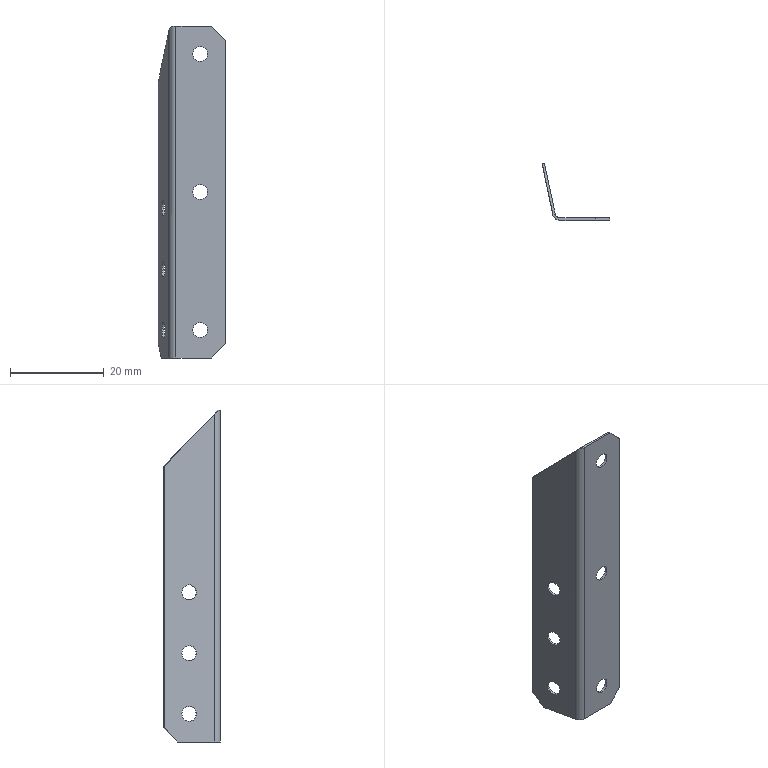Part | SolidWorks | features BaseBody 1 | 1 solid | 27 faces | box 14.467 x 12.157 x 71 mm | volume 767.375 mm3 | cylinder 14 | plane 12 | spline 1 | commonest cylinder face diameters 3.2 x12 2 x1 3 x1
STEP:
#1=CARTESIAN_POINT('',(6.25,-0.5,-27.9));
#2=VERTEX_POINT('',#1);
#3=CARTESIAN_POINT('',(6.25,-0.5,-31.1));
#4=VERTEX_POINT('',#3);
#5=CARTESIAN_POINT('',(6.25,-0.5,-29.5));
#6=DIRECTION('',(0.,-1.,0.));
#7=DIRECTION('',(0.,0.,1.));
#8=AXIS2_PLACEMENT_3D('',#5,#6,#7);
#9=CIRCLE('',#8,1.6);
#10=EDGE_CURVE('',#2,#4,#9,.T.);
#11=ORIENTED_EDGE('',*,*,#10,.T.);
#12=CARTESIAN_POINT('',(6.25,0.,-31.1));
#13=VERTEX_POINT('',#12);
#14=CARTESIAN_POINT('',(6.25,-0.5,-31.1));
#15=DIRECTION('',(0.,1.,0.));
#16=VECTOR('',#15,1000.);
#17=LINE('',#14,#16);
#18=EDGE_CURVE('',#4,#13,#17,.T.);
#19=ORIENTED_EDGE('',*,*,#18,.T.);
#20=CARTESIAN_POINT('',(6.25,0.,-27.9));
#21=VERTEX_POINT('',#20);
#22=CARTESIAN_POINT('',(6.25,0.,-29.5));
#23=DIRECTION('',(0.,1.,0.));
#24=DIRECTION('',(0.,0.,1.));
#25=AXIS2_PLACEMENT_3D('',#22,#23,#24);
#26=CIRCLE('',#25,1.6);
#27=EDGE_CURVE('',#13,#21,#26,.T.);
#28=ORIENTED_EDGE('',*,*,#27,.T.);
#29=CARTESIAN_POINT('',(6.25,-0.5,-27.9));
#30=DIRECTION('',(0.,1.,0.));
#31=VECTOR('',#30,1000.);
#32=LINE('',#29,#31);
#33=EDGE_CURVE('',#2,#21,#32,.T.);
#34=ORIENTED_EDGE('',*,*,#33,.F.);
#35=EDGE_LOOP('',(#11,#19,#28,#34));
#36=FACE_OUTER_BOUND('',#35,.T.);
#37=CARTESIAN_POINT('',(6.25,-0.5,-29.5));
#38=DIRECTION('',(0.,1.,0.));
#39=DIRECTION('',(0.,0.,1.));
#40=AXIS2_PLACEMENT_3D('',#37,#38,#39);
#41=CYLINDRICAL_SURFACE('',#40,1.6);
#42=ADVANCED_FACE('',(#36),#41,.F.);
#43=CARTESIAN_POINT('',(6.25,-0.5,1.6));
#44=VERTEX_POINT('',#43);
#45=CARTESIAN_POINT('',(6.25,-0.5,-1.6));
#46=VERTEX_POINT('',#45);
#47=CARTESIAN_POINT('',(6.25,-0.5,0.));
#48=DIRECTION('',(0.,-1.,0.));
#49=DIRECTION('',(0.,0.,1.));
#50=AXIS2_PLACEMENT_3D('',#47,#48,#49);
#51=CIRCLE('',#50,1.6);
#52=EDGE_CURVE('',#44,#46,#51,.T.);
#53=ORIENTED_EDGE('',*,*,#52,.T.);
#54=CARTESIAN_POINT('',(6.25,0.,-1.6));
#55=VERTEX_POINT('',#54);
#56=CARTESIAN_POINT('',(6.25,-0.5,-1.6));
#57=DIRECTION('',(0.,1.,0.));
#58=VECTOR('',#57,1000.);
#59=LINE('',#56,#58);
#60=EDGE_CURVE('',#46,#55,#59,.T.);
#61=ORIENTED_EDGE('',*,*,#60,.T.);
#62=CARTESIAN_POINT('',(6.25,0.,1.6));
#63=VERTEX_POINT('',#62);
#64=CARTESIAN_POINT('',(6.25,0.,0.));
#65=DIRECTION('',(0.,-1.,0.));
#66=DIRECTION('',(0.,0.,1.));
#67=AXIS2_PLACEMENT_3D('',#64,#65,#66);
#68=CIRCLE('',#67,1.6);
#69=EDGE_CURVE('',#63,#55,#68,.T.);
#70=ORIENTED_EDGE('',*,*,#69,.F.);
#71=CARTESIAN_POINT('',(6.25,-0.5,1.6));
#72=DIRECTION('',(0.,1.,0.));
#73=VECTOR('',#72,1000.);
#74=LINE('',#71,#73);
#75=EDGE_CURVE('',#44,#63,#74,.T.);
#76=ORIENTED_EDGE('',*,*,#75,.F.);
#77=EDGE_LOOP('',(#53,#61,#70,#76));
#78=FACE_OUTER_BOUND('',#77,.T.);
#79=CARTESIAN_POINT('',(6.25,-0.5,0.));
#80=DIRECTION('',(0.,1.,0.));
#81=DIRECTION('',(0.,0.,1.));
#82=AXIS2_PLACEMENT_3D('',#79,#80,#81);
#83=CYLINDRICAL_SURFACE('',#82,1.6);
#84=ADVANCED_FACE('',(#78),#83,.F.);
#85=CARTESIAN_POINT('',(6.25,-0.5,31.1));
#86=VERTEX_POINT('',#85);
#87=CARTESIAN_POINT('',(6.25,-0.5,27.9));
#88=VERTEX_POINT('',#87);
#89=CARTESIAN_POINT('',(6.25,-0.5,29.5));
#90=DIRECTION('',(0.,-1.,0.));
#91=DIRECTION('',(0.,0.,1.));
#92=AXIS2_PLACEMENT_3D('',#89,#90,#91);
#93=CIRCLE('',#92,1.6);
#94=EDGE_CURVE('',#86,#88,#93,.T.);
#95=ORIENTED_EDGE('',*,*,#94,.T.);
#96=CARTESIAN_POINT('',(6.25,0.,27.9));
#97=VERTEX_POINT('',#96);
#98=CARTESIAN_POINT('',(6.25,-0.5,27.9));
#99=DIRECTION('',(0.,1.,0.));
#100=VECTOR('',#99,1000.);
#101=LINE('',#98,#100);
#102=EDGE_CURVE('',#88,#97,#101,.T.);
#103=ORIENTED_EDGE('',*,*,#102,.T.);
#104=CARTESIAN_POINT('',(6.25,0.,31.1));
#105=VERTEX_POINT('',#104);
#106=CARTESIAN_POINT('',(6.25,0.,29.5));
#107=DIRECTION('',(0.,-1.,0.));
#108=DIRECTION('',(0.,0.,1.));
#109=AXIS2_PLACEMENT_3D('',#106,#107,#108);
#110=CIRCLE('',#109,1.6);
#111=EDGE_CURVE('',#105,#97,#110,.T.);
#112=ORIENTED_EDGE('',*,*,#111,.F.);
#113=CARTESIAN_POINT('',(6.25,-0.5,31.1));
#114=DIRECTION('',(0.,1.,0.));
#115=VECTOR('',#114,1000.);
#116=LINE('',#113,#115);
#117=EDGE_CURVE('',#86,#105,#116,.T.);
#118=ORIENTED_EDGE('',*,*,#117,.F.);
#119=EDGE_LOOP('',(#95,#103,#112,#118));
#120=FACE_OUTER_BOUND('',#119,.T.);
#121=CARTESIAN_POINT('',(6.25,-0.5,29.5));
#122=DIRECTION('',(0.,1.,0.));
#123=DIRECTION('',(0.,0.,1.));
#124=AXIS2_PLACEMENT_3D('',#121,#122,#123);
#125=CYLINDRICAL_SURFACE('',#124,1.6);
#126=ADVANCED_FACE('',(#120),#125,.F.);
#127=CARTESIAN_POINT('',(-1.906,7.739,-29.5));
#128=VERTEX_POINT('',#127);
#129=CARTESIAN_POINT('',(-1.241,4.609,-29.5));
#130=VERTEX_POINT('',#129);
#131=CARTESIAN_POINT('',(-1.573,6.174,-29.5));
#132=DIRECTION('',(-0.9781,-0.2079,0.));
#133=DIRECTION('',(-0.2079,0.9781,0.));
#134=AXIS2_PLACEMENT_3D('',#131,#132,#133);
#135=CIRCLE('',#134,1.6);
#136=EDGE_CURVE('',#128,#130,#135,.T.);
#137=ORIENTED_EDGE('',*,*,#136,.T.);
#138=CARTESIAN_POINT('',(-0.7517,4.713,-29.5));
#139=VERTEX_POINT('',#138);
#140=CARTESIAN_POINT('',(-1.241,4.609,-29.5));
#141=DIRECTION('',(0.9781,0.2079,0.));
#142=VECTOR('',#141,1000.);
#143=LINE('',#140,#142);
#144=EDGE_CURVE('',#130,#139,#143,.T.);
#145=ORIENTED_EDGE('',*,*,#144,.T.);
#146=CARTESIAN_POINT('',(-1.417,7.843,-29.5));
#147=VERTEX_POINT('',#146);
#148=CARTESIAN_POINT('',(-1.084,6.278,-29.5));
#149=DIRECTION('',(-0.9781,-0.2079,0.));
#150=DIRECTION('',(-0.2079,0.9781,0.));
#151=AXIS2_PLACEMENT_3D('',#148,#149,#150);
#152=CIRCLE('',#151,1.6);
#153=EDGE_CURVE('',#147,#139,#152,.T.);
#154=ORIENTED_EDGE('',*,*,#153,.F.);
#155=CARTESIAN_POINT('',(-1.906,7.739,-29.5));
#156=DIRECTION('',(0.9781,0.2079,0.));
#157=VECTOR('',#156,1000.);
#158=LINE('',#155,#157);
#159=EDGE_CURVE('',#128,#147,#158,.T.);
#160=ORIENTED_EDGE('',*,*,#159,.F.);
#161=EDGE_LOOP('',(#137,#145,#154,#160));
#162=FACE_OUTER_BOUND('',#161,.T.);
#163=CARTESIAN_POINT('',(-1.573,6.174,-29.5));
#164=DIRECTION('',(0.9781,0.2079,0.));
#165=DIRECTION('',(-0.2079,0.9781,0.));
#166=AXIS2_PLACEMENT_3D('',#163,#164,#165);
#167=CYLINDRICAL_SURFACE('',#166,1.6);
#168=ADVANCED_FACE('',(#162),#167,.F.);
#169=CARTESIAN_POINT('',(-1.906,7.739,-16.5));
#170=VERTEX_POINT('',#169);
#171=CARTESIAN_POINT('',(-1.241,4.609,-16.5));
#172=VERTEX_POINT('',#171);
#173=CARTESIAN_POINT('',(-1.573,6.174,-16.5));
#174=DIRECTION('',(-0.9781,-0.2079,0.));
#175=DIRECTION('',(-0.2079,0.9781,0.));
#176=AXIS2_PLACEMENT_3D('',#173,#174,#175);
#177=CIRCLE('',#176,1.6);
#178=EDGE_CURVE('',#170,#172,#177,.T.);
#179=ORIENTED_EDGE('',*,*,#178,.T.);
#180=CARTESIAN_POINT('',(-0.7517,4.713,-16.5));
#181=VERTEX_POINT('',#180);
#182=CARTESIAN_POINT('',(-1.241,4.609,-16.5));
#183=DIRECTION('',(0.9781,0.2079,0.));
#184=VECTOR('',#183,1000.);
#185=LINE('',#182,#184);
#186=EDGE_CURVE('',#172,#181,#185,.T.);
#187=ORIENTED_EDGE('',*,*,#186,.T.);
#188=CARTESIAN_POINT('',(-1.417,7.843,-16.5));
#189=VERTEX_POINT('',#188);
#190=CARTESIAN_POINT('',(-1.084,6.278,-16.5));
#191=DIRECTION('',(-0.9781,-0.2079,0.));
#192=DIRECTION('',(-0.2079,0.9781,0.));
#193=AXIS2_PLACEMENT_3D('',#190,#191,#192);
#194=CIRCLE('',#193,1.6);
#195=EDGE_CURVE('',#189,#181,#194,.T.);
#196=ORIENTED_EDGE('',*,*,#195,.F.);
#197=CARTESIAN_POINT('',(-1.906,7.739,-16.5));
#198=DIRECTION('',(0.9781,0.2079,0.));
#199=VECTOR('',#198,1000.);
#200=LINE('',#197,#199);
#201=EDGE_CURVE('',#170,#189,#200,.T.);
#202=ORIENTED_EDGE('',*,*,#201,.F.);
#203=EDGE_LOOP('',(#179,#187,#196,#202));
#204=FACE_OUTER_BOUND('',#203,.T.);
#205=CARTESIAN_POINT('',(-1.573,6.174,-16.5));
#206=DIRECTION('',(0.9781,0.2079,0.));
#207=DIRECTION('',(-0.2079,0.9781,0.));
#208=AXIS2_PLACEMENT_3D('',#205,#206,#207);
#209=CYLINDRICAL_SURFACE('',#208,1.6);
#210=ADVANCED_FACE('',(#204),#209,.F.);
#211=CARTESIAN_POINT('',(-1.906,7.739,-3.5));
#212=VERTEX_POINT('',#211);
#213=CARTESIAN_POINT('',(-1.241,4.609,-3.5));
#214=VERTEX_POINT('',#213);
#215=CARTESIAN_POINT('',(-1.573,6.174,-3.5));
#216=DIRECTION('',(-0.9781,-0.2079,0.));
#217=DIRECTION('',(-0.2079,0.9781,0.));
#218=AXIS2_PLACEMENT_3D('',#215,#216,#217);
#219=CIRCLE('',#218,1.6);
#220=EDGE_CURVE('',#212,#214,#219,.T.);
#221=ORIENTED_EDGE('',*,*,#220,.T.);
#222=CARTESIAN_POINT('',(-0.7517,4.713,-3.5));
#223=VERTEX_POINT('',#222);
#224=CARTESIAN_POINT('',(-1.241,4.609,-3.5));
#225=DIRECTION('',(0.9781,0.2079,0.));
#226=VECTOR('',#225,1000.);
#227=LINE('',#224,#226);
#228=EDGE_CURVE('',#214,#223,#227,.T.);
#229=ORIENTED_EDGE('',*,*,#228,.T.);
#230=CARTESIAN_POINT('',(-1.417,7.843,-3.5));
#231=VERTEX_POINT('',#230);
#232=CARTESIAN_POINT('',(-1.084,6.278,-3.5));
#233=DIRECTION('',(-0.9781,-0.2079,0.));
#234=DIRECTION('',(-0.2079,0.9781,0.));
#235=AXIS2_PLACEMENT_3D('',#232,#233,#234);
#236=CIRCLE('',#235,1.6);
#237=EDGE_CURVE('',#231,#223,#236,.T.);
#238=ORIENTED_EDGE('',*,*,#237,.F.);
#239=CARTESIAN_POINT('',(-1.906,7.739,-3.5));
#240=DIRECTION('',(0.9781,0.2079,0.));
#241=VECTOR('',#240,1000.);
#242=LINE('',#239,#241);
#243=EDGE_CURVE('',#212,#231,#242,.T.);
#244=ORIENTED_EDGE('',*,*,#243,.F.);
#245=EDGE_LOOP('',(#221,#229,#238,#244));
#246=FACE_OUTER_BOUND('',#245,.T.);
#247=CARTESIAN_POINT('',(-1.573,6.174,-3.5));
#248=DIRECTION('',(0.9781,0.2079,0.));
#249=DIRECTION('',(-0.2079,0.9781,0.));
#250=AXIS2_PLACEMENT_3D('',#247,#248,#249);
#251=CYLINDRICAL_SURFACE('',#250,1.6);
#252=ADVANCED_FACE('',(#246),#251,.F.);
#253=ORIENTED_EDGE('',*,*,#18,.F.);
#254=CARTESIAN_POINT('',(6.25,-0.5,-29.5));
#255=DIRECTION('',(0.,-1.,0.));
#256=DIRECTION('',(0.,0.,1.));
#257=AXIS2_PLACEMENT_3D('',#254,#255,#256);
#258=CIRCLE('',#257,1.6);
#259=EDGE_CURVE('',#4,#2,#258,.T.);
#260=ORIENTED_EDGE('',*,*,#259,.T.);
#261=ORIENTED_EDGE('',*,*,#33,.T.);
#262=CARTESIAN_POINT('',(6.25,0.,-29.5));
#263=DIRECTION('',(0.,1.,0.));
#264=DIRECTION('',(0.,0.,1.));
#265=AXIS2_PLACEMENT_3D('',#262,#263,#264);
#266=CIRCLE('',#265,1.6);
#267=EDGE_CURVE('',#21,#13,#266,.T.);
#268=ORIENTED_EDGE('',*,*,#267,.T.);
#269=EDGE_LOOP('',(#253,#260,#261,#268));
#270=FACE_OUTER_BOUND('',#269,.T.);
#271=CARTESIAN_POINT('',(6.25,-0.5,-29.5));
#272=DIRECTION('',(0.,1.,0.));
#273=DIRECTION('',(0.,0.,1.));
#274=AXIS2_PLACEMENT_3D('',#271,#272,#273);
#275=CYLINDRICAL_SURFACE('',#274,1.6);
#276=ADVANCED_FACE('',(#270),#275,.F.);
#277=ORIENTED_EDGE('',*,*,#267,.F.);
#278=ORIENTED_EDGE('',*,*,#27,.F.);
#279=EDGE_LOOP('',(#277,#278));
#280=FACE_BOUND('',#279,.T.);
#281=ORIENTED_EDGE('',*,*,#69,.T.);
#282=CARTESIAN_POINT('',(6.25,0.,0.));
#283=DIRECTION('',(0.,-1.,0.));
#284=DIRECTION('',(0.,0.,1.));
#285=AXIS2_PLACEMENT_3D('',#282,#283,#284);
#286=CIRCLE('',#285,1.6);
#287=EDGE_CURVE('',#55,#63,#286,.T.);
#288=ORIENTED_EDGE('',*,*,#287,.T.);
#289=EDGE_LOOP('',(#281,#288));
#290=FACE_BOUND('',#289,.T.);
#291=ORIENTED_EDGE('',*,*,#111,.T.);
#292=CARTESIAN_POINT('',(6.25,0.,29.5));
#293=DIRECTION('',(0.,-1.,0.));
#294=DIRECTION('',(0.,0.,1.));
#295=AXIS2_PLACEMENT_3D('',#292,#293,#294);
#296=CIRCLE('',#295,1.6);
#297=EDGE_CURVE('',#97,#105,#296,.T.);
#298=ORIENTED_EDGE('',*,*,#297,.T.);
#299=EDGE_LOOP('',(#291,#298));
#300=FACE_BOUND('',#299,.T.);
#301=CARTESIAN_POINT('',(11.75,0.,-32.5));
#302=VERTEX_POINT('',#301);
#303=CARTESIAN_POINT('',(8.75,0.,-35.5));
#304=VERTEX_POINT('',#303);
#305=CARTESIAN_POINT('',(11.75,0.,-32.5));
#306=DIRECTION('',(-0.7071,0.,-0.7071));
#307=VECTOR('',#306,1000.);
#308=LINE('',#305,#307);
#309=EDGE_CURVE('',#302,#304,#308,.T.);
#310=ORIENTED_EDGE('',*,*,#309,.T.);
#311=CARTESIAN_POINT('',(1.06,0.,-35.5));
#312=VERTEX_POINT('',#311);
#313=CARTESIAN_POINT('',(6.405,0.,-35.5));
#314=DIRECTION('',(-1.,0.,0.));
#315=VECTOR('',#314,1000.);
#316=LINE('',#313,#315);
#317=EDGE_CURVE('',#304,#312,#316,.T.);
#318=ORIENTED_EDGE('',*,*,#317,.T.);
#319=CARTESIAN_POINT('',(1.06,0.,35.5));
#320=VERTEX_POINT('',#319);
#321=CARTESIAN_POINT('',(1.06,0.,0.));
#322=DIRECTION('',(0.,0.,1.));
#323=VECTOR('',#322,1000.);
#324=LINE('',#321,#323);
#325=EDGE_CURVE('',#312,#320,#324,.T.);
#326=ORIENTED_EDGE('',*,*,#325,.T.);
#327=CARTESIAN_POINT('',(8.75,0.,35.5));
#328=VERTEX_POINT('',#327);
#329=CARTESIAN_POINT('',(6.405,0.,35.5));
#330=DIRECTION('',(1.,0.,0.));
#331=VECTOR('',#330,1000.);
#332=LINE('',#329,#331);
#333=EDGE_CURVE('',#320,#328,#332,.T.);
#334=ORIENTED_EDGE('',*,*,#333,.T.);
#335=CARTESIAN_POINT('',(11.75,0.,32.5));
#336=VERTEX_POINT('',#335);
#337=CARTESIAN_POINT('',(8.75,0.,35.5));
#338=DIRECTION('',(0.7071,0.,-0.7071));
#339=VECTOR('',#338,1000.);
#340=LINE('',#337,#339);
#341=EDGE_CURVE('',#328,#336,#340,.T.);
#342=ORIENTED_EDGE('',*,*,#341,.T.);
#343=CARTESIAN_POINT('',(11.75,0.,0.));
#344=DIRECTION('',(0.,0.,-1.));
#345=VECTOR('',#344,1000.);
#346=LINE('',#343,#345);
#347=EDGE_CURVE('',#336,#302,#346,.T.);
#348=ORIENTED_EDGE('',*,*,#347,.T.);
#349=EDGE_LOOP('',(#310,#318,#326,#334,#342,#348));
#350=FACE_OUTER_BOUND('',#349,.T.);
#351=CARTESIAN_POINT('',(11.75,0.,35.5));
#352=DIRECTION('',(0.,1.,0.));
#353=DIRECTION('',(0.,0.,-1.));
#354=AXIS2_PLACEMENT_3D('',#351,#352,#353);
#355=PLANE('',#354);
#356=ADVANCED_FACE('',(#280,#290,#300,#350),#355,.T.);
#357=ORIENTED_EDGE('',*,*,#94,.F.);
#358=CARTESIAN_POINT('',(6.25,-0.5,29.5));
#359=DIRECTION('',(0.,-1.,0.));
#360=DIRECTION('',(0.,0.,1.));
#361=AXIS2_PLACEMENT_3D('',#358,#359,#360);
#362=CIRCLE('',#361,1.6);
#363=EDGE_CURVE('',#88,#86,#362,.T.);
#364=ORIENTED_EDGE('',*,*,#363,.F.);
#365=EDGE_LOOP('',(#357,#364));
#366=FACE_BOUND('',#365,.T.);
#367=ORIENTED_EDGE('',*,*,#52,.F.);
#368=CARTESIAN_POINT('',(6.25,-0.5,0.));
#369=DIRECTION('',(0.,-1.,0.));
#370=DIRECTION('',(0.,0.,1.));
#371=AXIS2_PLACEMENT_3D('',#368,#369,#370);
#372=CIRCLE('',#371,1.6);
#373=EDGE_CURVE('',#46,#44,#372,.T.);
#374=ORIENTED_EDGE('',*,*,#373,.F.);
#375=EDGE_LOOP('',(#367,#374));
#376=FACE_BOUND('',#375,.T.);
#377=ORIENTED_EDGE('',*,*,#10,.F.);
#378=ORIENTED_EDGE('',*,*,#259,.F.);
#379=EDGE_LOOP('',(#377,#378));
#380=FACE_BOUND('',#379,.T.);
#381=CARTESIAN_POINT('',(11.75,-0.5,-32.5));
#382=VERTEX_POINT('',#381);
#383=CARTESIAN_POINT('',(8.75,-0.5,-35.5));
#384=VERTEX_POINT('',#383);
#385=CARTESIAN_POINT('',(8.75,-0.5,-35.5));
#386=DIRECTION('',(-0.7071,0.,-0.7071));
#387=VECTOR('',#386,1000.);
#388=LINE('',#385,#387);
#389=EDGE_CURVE('',#382,#384,#388,.T.);
#390=ORIENTED_EDGE('',*,*,#389,.F.);
#391=CARTESIAN_POINT('',(11.75,-0.5,32.5));
#392=VERTEX_POINT('',#391);
#393=CARTESIAN_POINT('',(11.75,-0.5,0.));
#394=DIRECTION('',(0.,0.,-1.));
#395=VECTOR('',#394,1000.);
#396=LINE('',#393,#395);
#397=EDGE_CURVE('',#392,#382,#396,.T.);
#398=ORIENTED_EDGE('',*,*,#397,.F.);
#399=CARTESIAN_POINT('',(8.75,-0.5,35.5));
#400=VERTEX_POINT('',#399);
#401=CARTESIAN_POINT('',(11.75,-0.5,32.5));
#402=DIRECTION('',(0.7071,0.,-0.7071));
#403=VECTOR('',#402,1000.);
#404=LINE('',#401,#403);
#405=EDGE_CURVE('',#400,#392,#404,.T.);
#406=ORIENTED_EDGE('',*,*,#405,.F.);
#407=CARTESIAN_POINT('',(1.06,-0.5,35.5));
#408=VERTEX_POINT('',#407);
#409=CARTESIAN_POINT('',(6.405,-0.5,35.5));
#410=DIRECTION('',(1.,0.,0.));
#411=VECTOR('',#410,1000.);
#412=LINE('',#409,#411);
#413=EDGE_CURVE('',#408,#400,#412,.T.);
#414=ORIENTED_EDGE('',*,*,#413,.F.);
#415=CARTESIAN_POINT('',(1.06,-0.5,-35.5));
#416=VERTEX_POINT('',#415);
#417=CARTESIAN_POINT('',(1.06,-0.5,0.));
#418=DIRECTION('',(0.,0.,1.));
#419=VECTOR('',#418,1000.);
#420=LINE('',#417,#419);
#421=EDGE_CURVE('',#416,#408,#420,.T.);
#422=ORIENTED_EDGE('',*,*,#421,.F.);
#423=CARTESIAN_POINT('',(6.405,-0.5,-35.5));
#424=DIRECTION('',(-1.,0.,0.));
#425=VECTOR('',#424,1000.);
#426=LINE('',#423,#425);
#427=EDGE_CURVE('',#384,#416,#426,.T.);
#428=ORIENTED_EDGE('',*,*,#427,.F.);
#429=EDGE_LOOP('',(#390,#398,#406,#414,#422,#428));
#430=FACE_OUTER_BOUND('',#429,.T.);
#431=CARTESIAN_POINT('',(11.75,-0.5,35.5));
#432=DIRECTION('',(0.,1.,0.));
#433=DIRECTION('',(0.,0.,-1.));
#434=AXIS2_PLACEMENT_3D('',#431,#432,#433);
#435=PLANE('',#434);
#436=ADVANCED_FACE('',(#366,#376,#380,#430),#435,.F.);
#437=ORIENTED_EDGE('',*,*,#60,.F.);
#438=ORIENTED_EDGE('',*,*,#373,.T.);
#439=ORIENTED_EDGE('',*,*,#75,.T.);
#440=ORIENTED_EDGE('',*,*,#287,.F.);
#441=EDGE_LOOP('',(#437,#438,#439,#440));
#442=FACE_OUTER_BOUND('',#441,.T.);
#443=CARTESIAN_POINT('',(6.25,-0.5,0.));
#444=DIRECTION('',(0.,1.,0.));
#445=DIRECTION('',(0.,0.,1.));
#446=AXIS2_PLACEMENT_3D('',#443,#444,#445);
#447=CYLINDRICAL_SURFACE('',#446,1.6);
#448=ADVANCED_FACE('',(#442),#447,.F.);
#449=ORIENTED_EDGE('',*,*,#102,.F.);
#450=ORIENTED_EDGE('',*,*,#363,.T.);
#451=ORIENTED_EDGE('',*,*,#117,.T.);
#452=ORIENTED_EDGE('',*,*,#297,.F.);
#453=EDGE_LOOP('',(#449,#450,#451,#452));
#454=FACE_OUTER_BOUND('',#453,.T.);
#455=CARTESIAN_POINT('',(6.25,-0.5,29.5));
#456=DIRECTION('',(0.,1.,0.));
#457=DIRECTION('',(0.,0.,1.));
#458=AXIS2_PLACEMENT_3D('',#455,#456,#457);
#459=CYLINDRICAL_SURFACE('',#458,1.6);
#460=ADVANCED_FACE('',(#454),#459,.F.);
#461=CARTESIAN_POINT('',(8.75,-0.25,-35.5));
#462=DIRECTION('',(0.,-1.,0.));
#463=VECTOR('',#462,1000.);
#464=LINE('',#461,#463);
#465=EDGE_CURVE('',#304,#384,#464,.T.);
#466=ORIENTED_EDGE('',*,*,#465,.T.);
#467=ORIENTED_EDGE('',*,*,#427,.T.);
#468=CARTESIAN_POINT('',(-0.4074,0.6881,-35.5));
#469=VERTEX_POINT('',#468);
#470=CARTESIAN_POINT('',(1.06,1.,-35.5));
#471=DIRECTION('',(0.,0.,-1.));
#472=DIRECTION('',(1.,0.,0.));
#473=AXIS2_PLACEMENT_3D('',#470,#471,#472);
#474=CIRCLE('',#473,1.5);
#475=EDGE_CURVE('',#416,#469,#474,.T.);
#476=ORIENTED_EDGE('',*,*,#475,.T.);
#477=CARTESIAN_POINT('',(-2.093,8.619,-35.5));
#478=VERTEX_POINT('',#477);
#479=CARTESIAN_POINT('',(-1.562,6.121,-35.5));
#480=DIRECTION('',(-0.2079,0.9781,0.));
#481=VECTOR('',#480,1000.);
#482=LINE('',#479,#481);
#483=EDGE_CURVE('',#469,#478,#482,.T.);
#484=ORIENTED_EDGE('',*,*,#483,.T.);
#485=CARTESIAN_POINT('',(-1.604,8.723,-35.5));
#486=VERTEX_POINT('',#485);
#487=CARTESIAN_POINT('',(-1.849,8.671,-35.5));
#488=DIRECTION('',(-0.9781,-0.2079,0.));
#489=VECTOR('',#488,1000.);
#490=LINE('',#487,#489);
#491=EDGE_CURVE('',#486,#478,#490,.T.);
#492=ORIENTED_EDGE('',*,*,#491,.F.);
#493=CARTESIAN_POINT('',(0.08164,0.7921,-35.5));
#494=VERTEX_POINT('',#493);
#495=CARTESIAN_POINT('',(-1.073,6.225,-35.5));
#496=DIRECTION('',(-0.2079,0.9781,0.));
#497=VECTOR('',#496,1000.);
#498=LINE('',#495,#497);
#499=EDGE_CURVE('',#494,#486,#498,.T.);
#500=ORIENTED_EDGE('',*,*,#499,.F.);
#501=CARTESIAN_POINT('',(1.06,1.,-35.5));
#502=DIRECTION('',(0.,0.,1.));
#503=DIRECTION('',(1.,0.,0.));
#504=AXIS2_PLACEMENT_3D('',#501,#502,#503);
#505=CIRCLE('',#504,1.);
#506=EDGE_CURVE('',#494,#312,#505,.T.);
#507=ORIENTED_EDGE('',*,*,#506,.T.);
#508=ORIENTED_EDGE('',*,*,#317,.F.);
#509=EDGE_LOOP('',(#466,#467,#476,#484,#492,#500,#507,#508));
#510=FACE_OUTER_BOUND('',#509,.T.);
#511=CARTESIAN_POINT('',(1.06,0.,-35.5));
#512=DIRECTION('',(0.,0.,-1.));
#513=DIRECTION('',(1.,0.,0.));
#514=AXIS2_PLACEMENT_3D('',#511,#512,#513);
#515=PLANE('',#514);
#516=ADVANCED_FACE('',(#510),#515,.T.);
#517=ORIENTED_EDGE('',*,*,#389,.T.);
#518=ORIENTED_EDGE('',*,*,#465,.F.);
#519=ORIENTED_EDGE('',*,*,#309,.F.);
#520=CARTESIAN_POINT('',(11.75,-0.25,-32.5));
#521=DIRECTION('',(0.,-1.,0.));
#522=VECTOR('',#521,1000.);
#523=LINE('',#520,#522);
#524=EDGE_CURVE('',#302,#382,#523,.T.);
#525=ORIENTED_EDGE('',*,*,#524,.T.);
#526=EDGE_LOOP('',(#517,#518,#519,#525));
#527=FACE_OUTER_BOUND('',#526,.T.);
#528=CARTESIAN_POINT('',(8.75,0.,-35.5));
#529=DIRECTION('',(0.7071,0.,-0.7071));
#530=DIRECTION('',(0.7071,0.,0.7071));
#531=AXIS2_PLACEMENT_3D('',#528,#529,#530);
#532=PLANE('',#531);
#533=ADVANCED_FACE('',(#527),#532,.T.);
#534=ORIENTED_EDGE('',*,*,#397,.T.);
#535=ORIENTED_EDGE('',*,*,#524,.F.);
#536=ORIENTED_EDGE('',*,*,#347,.F.);
#537=CARTESIAN_POINT('',(11.75,-0.25,32.5));
#538=DIRECTION('',(0.,-1.,0.));
#539=VECTOR('',#538,1000.);
#540=LINE('',#537,#539);
#541=EDGE_CURVE('',#336,#392,#540,.T.);
#542=ORIENTED_EDGE('',*,*,#541,.T.);
#543=EDGE_LOOP('',(#534,#535,#536,#542));
#544=FACE_OUTER_BOUND('',#543,.T.);
#545=CARTESIAN_POINT('',(11.75,0.,-32.5));
#546=DIRECTION('',(1.,0.,0.));
#547=DIRECTION('',(0.,0.,1.));
#548=AXIS2_PLACEMENT_3D('',#545,#546,#547);
#549=PLANE('',#548);
#550=ADVANCED_FACE('',(#544),#549,.T.);
#551=ORIENTED_EDGE('',*,*,#405,.T.);
#552=ORIENTED_EDGE('',*,*,#541,.F.);
#553=ORIENTED_EDGE('',*,*,#341,.F.);
#554=CARTESIAN_POINT('',(8.75,-0.25,35.5));
#555=DIRECTION('',(0.,-1.,0.));
#556=VECTOR('',#555,1000.);
#557=LINE('',#554,#556);
#558=EDGE_CURVE('',#328,#400,#557,.T.);
#559=ORIENTED_EDGE('',*,*,#558,.T.);
#560=EDGE_LOOP('',(#551,#552,#553,#559));
#561=FACE_OUTER_BOUND('',#560,.T.);
#562=CARTESIAN_POINT('',(11.75,0.,32.5));
#563=DIRECTION('',(0.7071,0.,0.7071));
#564=DIRECTION('',(-0.7071,0.,0.7071));
#565=AXIS2_PLACEMENT_3D('',#562,#563,#564);
#566=PLANE('',#565);
#567=ADVANCED_FACE('',(#561),#566,.T.);
#568=ORIENTED_EDGE('',*,*,#558,.F.);
#569=ORIENTED_EDGE('',*,*,#333,.F.);
#570=CARTESIAN_POINT('',(0.4563,0.2026,35.5));
#571=VERTEX_POINT('',#570);
#572=CARTESIAN_POINT('',(1.06,1.,35.5));
#573=DIRECTION('',(0.,0.,1.));
#574=DIRECTION('',(1.,0.,0.));
#575=AXIS2_PLACEMENT_3D('',#572,#573,#574);
#576=CIRCLE('',#575,1.);
#577=EDGE_CURVE('',#571,#320,#576,.T.);
#578=ORIENTED_EDGE('',*,*,#577,.F.);
#579=CARTESIAN_POINT('',(0.1546,-0.1961,35.5));
#580=VERTEX_POINT('',#579);
#581=CARTESIAN_POINT('',(0.4563,0.2026,35.5));
#582=DIRECTION('',(-0.6035,-0.7974,0.));
#583=VECTOR('',#582,1000.);
#584=LINE('',#581,#583);
#585=EDGE_CURVE('',#571,#580,#584,.T.);
#586=ORIENTED_EDGE('',*,*,#585,.T.);
#587=CARTESIAN_POINT('',(1.06,1.,35.5));
#588=DIRECTION('',(0.,0.,1.));
#589=DIRECTION('',(1.,0.,0.));
#590=AXIS2_PLACEMENT_3D('',#587,#588,#589);
#591=CIRCLE('',#590,1.5);
#592=EDGE_CURVE('',#580,#408,#591,.T.);
#593=ORIENTED_EDGE('',*,*,#592,.T.);
#594=ORIENTED_EDGE('',*,*,#413,.T.);
#595=EDGE_LOOP('',(#568,#569,#578,#586,#593,#594));
#596=FACE_OUTER_BOUND('',#595,.T.);
#597=CARTESIAN_POINT('',(8.75,0.,35.5));
#598=DIRECTION('',(0.,0.,1.));
#599=DIRECTION('',(-1.,0.,0.));
#600=AXIS2_PLACEMENT_3D('',#597,#598,#599);
#601=PLANE('',#600);
#602=ADVANCED_FACE('',(#596),#601,.T.);
#603=CARTESIAN_POINT('',(0.08164,0.7921,34.608));
#604=VERTEX_POINT('',#603);
#605=CARTESIAN_POINT('',(0.08164,0.7921,0.));
#606=DIRECTION('',(0.,0.,1.));
#607=VECTOR('',#606,1000.);
#608=LINE('',#605,#607);
#609=EDGE_CURVE('',#494,#604,#608,.T.);
#610=ORIENTED_EDGE('',*,*,#609,.T.);
#611=CARTESIAN_POINT('',(0.08164,0.7921,34.608));
#612=CARTESIAN_POINT('',(0.1312,0.559,34.906));
#613=CARTESIAN_POINT('',(0.2663,0.3464,35.202));
#614=CARTESIAN_POINT('',(0.4563,0.2026,35.5));
#615=B_SPLINE_CURVE_WITH_KNOTS('',3,(#611,#612,#613,#614),.UNSPECIFIED.,.F.,.F.,(4,4),(0.,0.00114),.UNSPECIFIED.);
#616=EDGE_CURVE('',#604,#571,#615,.T.);
#617=ORIENTED_EDGE('',*,*,#616,.T.);
#618=ORIENTED_EDGE('',*,*,#577,.T.);
#619=ORIENTED_EDGE('',*,*,#325,.F.);
#620=ORIENTED_EDGE('',*,*,#506,.F.);
#621=EDGE_LOOP('',(#610,#617,#618,#619,#620));
#622=FACE_OUTER_BOUND('',#621,.T.);
#623=CARTESIAN_POINT('',(1.06,1.,-35.5));
#624=DIRECTION('',(0.,0.,1.));
#625=DIRECTION('',(1.,0.,0.));
#626=AXIS2_PLACEMENT_3D('',#623,#624,#625);
#627=CYLINDRICAL_SURFACE('',#626,1.);
#628=ADVANCED_FACE('',(#622),#627,.F.);
#629=CARTESIAN_POINT('',(-0.4074,0.6881,34.608));
#630=VERTEX_POINT('',#629);
#631=CARTESIAN_POINT('',(-0.4074,0.6881,34.608));
#632=CARTESIAN_POINT('',(-0.3702,0.5131,34.757));
#633=CARTESIAN_POINT('',(-0.3017,0.3456,34.906));
#634=CARTESIAN_POINT('',(-0.1103,0.04463,35.203));
#635=CARTESIAN_POINT('',(0.01194,-0.08813,35.351));
#636=CARTESIAN_POINT('',(0.1546,-0.1961,35.5));
#637=B_SPLINE_CURVE_WITH_KNOTS('',3,(#631,#632,#633,#634,#635,#636),.UNSPECIFIED.,.F.,.F.,(4,2,4),(0.,0.0006962,0.001392),.UNSPECIFIED.);
#638=EDGE_CURVE('',#630,#580,#637,.T.);
#639=ORIENTED_EDGE('',*,*,#638,.F.);
#640=CARTESIAN_POINT('',(-0.4074,0.6881,0.));
#641=DIRECTION('',(0.,0.,1.));
#642=VECTOR('',#641,1000.);
#643=LINE('',#640,#642);
#644=EDGE_CURVE('',#469,#630,#643,.T.);
#645=ORIENTED_EDGE('',*,*,#644,.F.);
#646=ORIENTED_EDGE('',*,*,#475,.F.);
#647=ORIENTED_EDGE('',*,*,#421,.T.);
#648=ORIENTED_EDGE('',*,*,#592,.F.);
#649=EDGE_LOOP('',(#639,#645,#646,#647,#648));
#650=FACE_OUTER_BOUND('',#649,.T.);
#651=CARTESIAN_POINT('',(1.06,1.,-35.5));
#652=DIRECTION('',(0.,0.,1.));
#653=DIRECTION('',(1.,0.,0.));
#654=AXIS2_PLACEMENT_3D('',#651,#652,#653);
#655=CYLINDRICAL_SURFACE('',#654,1.5);
#656=ADVANCED_FACE('',(#650),#655,.T.);
#657=ORIENTED_EDGE('',*,*,#638,.T.);
#658=ORIENTED_EDGE('',*,*,#585,.F.);
#659=ORIENTED_EDGE('',*,*,#616,.F.);
#660=CARTESIAN_POINT('',(-0.1629,0.7401,34.608));
#661=DIRECTION('',(0.9781,0.2079,0.));
#662=VECTOR('',#661,1000.);
#663=LINE('',#660,#662);
#664=EDGE_CURVE('',#630,#604,#663,.T.);
#665=ORIENTED_EDGE('',*,*,#664,.F.);
#666=EDGE_LOOP('',(#657,#658,#659,#665));
#667=FACE_OUTER_BOUND('',#666,.T.);
#668=CARTESIAN_POINT('',(-0.4124,0.6871,34.608));
#669=CARTESIAN_POINT('',(-0.3752,0.512,34.757));
#670=CARTESIAN_POINT('',(-0.3064,0.3437,34.905));
#671=CARTESIAN_POINT('',(-0.1144,0.04159,35.203));
#672=CARTESIAN_POINT('',(0.008823,-0.09211,35.351));
#673=CARTESIAN_POINT('',(0.1516,-0.2001,35.5));
#674=CARTESIAN_POINT('',(-0.4074,0.6881,34.608));
#675=CARTESIAN_POINT('',(-0.3703,0.5136,34.757));
#676=CARTESIAN_POINT('',(-0.3018,0.3459,34.905));
#677=CARTESIAN_POINT('',(-0.1104,0.04481,35.203));
#678=CARTESIAN_POINT('',(0.01235,-0.08844,35.351));
#679=CARTESIAN_POINT('',(0.1546,-0.1961,35.5));
#680=CARTESIAN_POINT('',(0.08164,0.7921,34.608));
#681=CARTESIAN_POINT('',(0.1064,0.6758,34.757));
#682=CARTESIAN_POINT('',(0.152,0.5639,34.905));
#683=CARTESIAN_POINT('',(0.2796,0.3632,35.203));
#684=CARTESIAN_POINT('',(0.3615,0.2744,35.351));
#685=CARTESIAN_POINT('',(0.4563,0.2026,35.5));
#686=CARTESIAN_POINT('',(0.08653,0.7931,34.608));
#687=CARTESIAN_POINT('',(0.1111,0.6774,34.757));
#688=CARTESIAN_POINT('',(0.1566,0.5661,34.905));
#689=CARTESIAN_POINT('',(0.2835,0.3664,35.203));
#690=CARTESIAN_POINT('',(0.365,0.278,35.351));
#691=CARTESIAN_POINT('',(0.4593,0.2066,35.5));
#692=B_SPLINE_SURFACE_WITH_KNOTS('',1,3,((#668,#669,#670,#671,#672,#673),(#674,#675,#676,#677,#678,#679),(#680,#681,#682,#683,#684,#685),(#686,#687,#688,#689,#690,#691)),.UNSPECIFIED.,.F.,.F.,.F.,(2,1,1,2),(4,2,4),(-0.0101,0.,1.,1.01),(0.,0.5,1.),.UNSPECIFIED.);
#693=ADVANCED_FACE('',(#667),#692,.F.);
#694=ORIENTED_EDGE('',*,*,#153,.T.);
#695=CARTESIAN_POINT('',(-1.084,6.278,-29.5));
#696=DIRECTION('',(-0.9781,-0.2079,0.));
#697=DIRECTION('',(-0.2079,0.9781,0.));
#698=AXIS2_PLACEMENT_3D('',#695,#696,#697);
#699=CIRCLE('',#698,1.6);
#700=EDGE_CURVE('',#139,#147,#699,.T.);
#701=ORIENTED_EDGE('',*,*,#700,.T.);
#702=EDGE_LOOP('',(#694,#701));
#703=FACE_BOUND('',#702,.T.);
#704=ORIENTED_EDGE('',*,*,#195,.T.);
#705=CARTESIAN_POINT('',(-1.084,6.278,-16.5));
#706=DIRECTION('',(-0.9781,-0.2079,0.));
#707=DIRECTION('',(-0.2079,0.9781,0.));
#708=AXIS2_PLACEMENT_3D('',#705,#706,#707);
#709=CIRCLE('',#708,1.6);
#710=EDGE_CURVE('',#181,#189,#709,.T.);
#711=ORIENTED_EDGE('',*,*,#710,.T.);
#712=EDGE_LOOP('',(#704,#711));
#713=FACE_BOUND('',#712,.T.);
#714=ORIENTED_EDGE('',*,*,#237,.T.);
#715=CARTESIAN_POINT('',(-1.084,6.278,-3.5));
#716=DIRECTION('',(-0.9781,-0.2079,0.));
#717=DIRECTION('',(-0.2079,0.9781,0.));
#718=AXIS2_PLACEMENT_3D('',#715,#716,#717);
#719=CIRCLE('',#718,1.6);
#720=EDGE_CURVE('',#223,#231,#719,.T.);
#721=ORIENTED_EDGE('',*,*,#720,.T.);
#722=EDGE_LOOP('',(#714,#721));
#723=FACE_BOUND('',#722,.T.);
#724=CARTESIAN_POINT('',(-2.228,11.657,23.5));
#725=VERTEX_POINT('',#724);
#726=CARTESIAN_POINT('',(-2.228,11.657,23.5));
#727=DIRECTION('',(0.147,-0.6917,0.7071));
#728=VECTOR('',#727,1000.);
#729=LINE('',#726,#728);
#730=EDGE_CURVE('',#725,#604,#729,.T.);
#731=ORIENTED_EDGE('',*,*,#730,.T.);
#732=ORIENTED_EDGE('',*,*,#609,.F.);
#733=ORIENTED_EDGE('',*,*,#499,.T.);
#734=CARTESIAN_POINT('',(-2.228,11.657,-32.5));
#735=VERTEX_POINT('',#734);
#736=CARTESIAN_POINT('',(-1.604,8.723,-35.5));
#737=DIRECTION('',(-0.147,0.6917,0.7071));
#738=VECTOR('',#737,1000.);
#739=LINE('',#736,#738);
#740=EDGE_CURVE('',#486,#735,#739,.T.);
#741=ORIENTED_EDGE('',*,*,#740,.T.);
#742=CARTESIAN_POINT('',(-2.228,11.657,-0.2356));
#743=DIRECTION('',(0.,0.,1.));
#744=VECTOR('',#743,1000.);
#745=LINE('',#742,#744);
#746=EDGE_CURVE('',#735,#725,#745,.T.);
#747=ORIENTED_EDGE('',*,*,#746,.T.);
#748=EDGE_LOOP('',(#731,#732,#733,#741,#747));
#749=FACE_OUTER_BOUND('',#748,.T.);
#750=CARTESIAN_POINT('',(0.08164,0.7921,35.029));
#751=DIRECTION('',(0.9781,0.2079,0.));
#752=DIRECTION('',(0.,0.,-1.));
#753=AXIS2_PLACEMENT_3D('',#750,#751,#752);
#754=PLANE('',#753);
#755=ADVANCED_FACE('',(#703,#713,#723,#749),#754,.T.);
#756=ORIENTED_EDGE('',*,*,#220,.F.);
#757=CARTESIAN_POINT('',(-1.573,6.174,-3.5));
#758=DIRECTION('',(-0.9781,-0.2079,0.));
#759=DIRECTION('',(-0.2079,0.9781,0.));
#760=AXIS2_PLACEMENT_3D('',#757,#758,#759);
#761=CIRCLE('',#760,1.6);
#762=EDGE_CURVE('',#214,#212,#761,.T.);
#763=ORIENTED_EDGE('',*,*,#762,.F.);
#764=EDGE_LOOP('',(#756,#763));
#765=FACE_BOUND('',#764,.T.);
#766=ORIENTED_EDGE('',*,*,#178,.F.);
#767=CARTESIAN_POINT('',(-1.573,6.174,-16.5));
#768=DIRECTION('',(-0.9781,-0.2079,0.));
#769=DIRECTION('',(-0.2079,0.9781,0.));
#770=AXIS2_PLACEMENT_3D('',#767,#768,#769);
#771=CIRCLE('',#770,1.6);
#772=EDGE_CURVE('',#172,#170,#771,.T.);
#773=ORIENTED_EDGE('',*,*,#772,.F.);
#774=EDGE_LOOP('',(#766,#773));
#775=FACE_BOUND('',#774,.T.);
#776=ORIENTED_EDGE('',*,*,#136,.F.);
#777=CARTESIAN_POINT('',(-1.573,6.174,-29.5));
#778=DIRECTION('',(-0.9781,-0.2079,0.));
#779=DIRECTION('',(-0.2079,0.9781,0.));
#780=AXIS2_PLACEMENT_3D('',#777,#778,#779);
#781=CIRCLE('',#780,1.6);
#782=EDGE_CURVE('',#130,#128,#781,.T.);
#783=ORIENTED_EDGE('',*,*,#782,.F.);
#784=EDGE_LOOP('',(#776,#783));
#785=FACE_BOUND('',#784,.T.);
#786=CARTESIAN_POINT('',(-2.717,11.553,23.5));
#787=VERTEX_POINT('',#786);
#788=CARTESIAN_POINT('',(-0.4074,0.6881,34.608));
#789=DIRECTION('',(0.147,-0.6917,0.7071));
#790=VECTOR('',#789,1000.);
#791=LINE('',#788,#790);
#792=EDGE_CURVE('',#787,#630,#791,.T.);
#793=ORIENTED_EDGE('',*,*,#792,.F.);
#794=CARTESIAN_POINT('',(-2.717,11.553,-32.5));
#795=VERTEX_POINT('',#794);
#796=CARTESIAN_POINT('',(-2.717,11.553,-0.2356));
#797=DIRECTION('',(0.,0.,1.));
#798=VECTOR('',#797,1000.);
#799=LINE('',#796,#798);
#800=EDGE_CURVE('',#795,#787,#799,.T.);
#801=ORIENTED_EDGE('',*,*,#800,.F.);
#802=CARTESIAN_POINT('',(-2.717,11.553,-32.5));
#803=DIRECTION('',(-0.147,0.6917,0.7071));
#804=VECTOR('',#803,1000.);
#805=LINE('',#802,#804);
#806=EDGE_CURVE('',#478,#795,#805,.T.);
#807=ORIENTED_EDGE('',*,*,#806,.F.);
#808=ORIENTED_EDGE('',*,*,#483,.F.);
#809=ORIENTED_EDGE('',*,*,#644,.T.);
#810=EDGE_LOOP('',(#793,#801,#807,#808,#809));
#811=FACE_OUTER_BOUND('',#810,.T.);
#812=CARTESIAN_POINT('',(-0.4074,0.6881,35.029));
#813=DIRECTION('',(0.9781,0.2079,0.));
#814=DIRECTION('',(0.,0.,-1.));
#815=AXIS2_PLACEMENT_3D('',#812,#813,#814);
#816=PLANE('',#815);
#817=ADVANCED_FACE('',(#765,#775,#785,#811),#816,.F.);
#818=ORIENTED_EDGE('',*,*,#144,.F.);
#819=ORIENTED_EDGE('',*,*,#782,.T.);
#820=ORIENTED_EDGE('',*,*,#159,.T.);
#821=ORIENTED_EDGE('',*,*,#700,.F.);
#822=EDGE_LOOP('',(#818,#819,#820,#821));
#823=FACE_OUTER_BOUND('',#822,.T.);
#824=CARTESIAN_POINT('',(-1.573,6.174,-29.5));
#825=DIRECTION('',(0.9781,0.2079,0.));
#826=DIRECTION('',(-0.2079,0.9781,0.));
#827=AXIS2_PLACEMENT_3D('',#824,#825,#826);
#828=CYLINDRICAL_SURFACE('',#827,1.6);
#829=ADVANCED_FACE('',(#823),#828,.F.);
#830=ORIENTED_EDGE('',*,*,#186,.F.);
#831=ORIENTED_EDGE('',*,*,#772,.T.);
#832=ORIENTED_EDGE('',*,*,#201,.T.);
#833=ORIENTED_EDGE('',*,*,#710,.F.);
#834=EDGE_LOOP('',(#830,#831,#832,#833));
#835=FACE_OUTER_BOUND('',#834,.T.);
#836=CARTESIAN_POINT('',(-1.573,6.174,-16.5));
#837=DIRECTION('',(0.9781,0.2079,0.));
#838=DIRECTION('',(-0.2079,0.9781,0.));
#839=AXIS2_PLACEMENT_3D('',#836,#837,#838);
#840=CYLINDRICAL_SURFACE('',#839,1.6);
#841=ADVANCED_FACE('',(#835),#840,.F.);
#842=ORIENTED_EDGE('',*,*,#228,.F.);
#843=ORIENTED_EDGE('',*,*,#762,.T.);
#844=ORIENTED_EDGE('',*,*,#243,.T.);
#845=ORIENTED_EDGE('',*,*,#720,.F.);
#846=EDGE_LOOP('',(#842,#843,#844,#845));
#847=FACE_OUTER_BOUND('',#846,.T.);
#848=CARTESIAN_POINT('',(-1.573,6.174,-3.5));
#849=DIRECTION('',(0.9781,0.2079,0.));
#850=DIRECTION('',(-0.2079,0.9781,0.));
#851=AXIS2_PLACEMENT_3D('',#848,#849,#850);
#852=CYLINDRICAL_SURFACE('',#851,1.6);
#853=ADVANCED_FACE('',(#847),#852,.F.);
#854=ORIENTED_EDGE('',*,*,#792,.T.);
#855=ORIENTED_EDGE('',*,*,#664,.T.);
#856=ORIENTED_EDGE('',*,*,#730,.F.);
#857=CARTESIAN_POINT('',(-2.472,11.605,23.5));
#858=DIRECTION('',(-0.9781,-0.2079,0.));
#859=VECTOR('',#858,1000.);
#860=LINE('',#857,#859);
#861=EDGE_CURVE('',#725,#787,#860,.T.);
#862=ORIENTED_EDGE('',*,*,#861,.T.);
#863=EDGE_LOOP('',(#854,#855,#856,#862));
#864=FACE_OUTER_BOUND('',#863,.T.);
#865=CARTESIAN_POINT('',(0.08164,0.7921,34.608));
#866=DIRECTION('',(-0.147,0.6917,0.7071));
#867=DIRECTION('',(-0.147,0.6917,-0.7071));
#868=AXIS2_PLACEMENT_3D('',#865,#866,#867);
#869=PLANE('',#868);
#870=ADVANCED_FACE('',(#864),#869,.T.);
#871=ORIENTED_EDGE('',*,*,#800,.T.);
#872=ORIENTED_EDGE('',*,*,#861,.F.);
#873=ORIENTED_EDGE('',*,*,#746,.F.);
#874=CARTESIAN_POINT('',(-2.472,11.605,-32.5));
#875=DIRECTION('',(-0.9781,-0.2079,0.));
#876=VECTOR('',#875,1000.);
#877=LINE('',#874,#876);
#878=EDGE_CURVE('',#735,#795,#877,.T.);
#879=ORIENTED_EDGE('',*,*,#878,.T.);
#880=EDGE_LOOP('',(#871,#872,#873,#879));
#881=FACE_OUTER_BOUND('',#880,.T.);
#882=CARTESIAN_POINT('',(-2.228,11.657,23.5));
#883=DIRECTION('',(-0.2079,0.9781,0.));
#884=DIRECTION('',(0.,0.,-1.));
#885=AXIS2_PLACEMENT_3D('',#882,#883,#884);
#886=PLANE('',#885);
#887=ADVANCED_FACE('',(#881),#886,.T.);
#888=ORIENTED_EDGE('',*,*,#806,.T.);
#889=ORIENTED_EDGE('',*,*,#878,.F.);
#890=ORIENTED_EDGE('',*,*,#740,.F.);
#891=ORIENTED_EDGE('',*,*,#491,.T.);
#892=EDGE_LOOP('',(#888,#889,#890,#891));
#893=FACE_OUTER_BOUND('',#892,.T.);
#894=CARTESIAN_POINT('',(-2.228,11.657,-32.5));
#895=DIRECTION('',(-0.147,0.6917,-0.7071));
#896=DIRECTION('',(0.147,-0.6917,-0.7071));
#897=AXIS2_PLACEMENT_3D('',#894,#895,#896);
#898=PLANE('',#897);
#899=ADVANCED_FACE('',(#893),#898,.T.);
#900=CLOSED_SHELL('',(#42,#84,#126,#168,#210,#252,#276,#356,#436,#448,#460,#516,#533,#550,#567,#602,#628,#656,#693,#755,#817,#829,#841,#853,#870,#887,#899));
#901=MANIFOLD_SOLID_BREP('',#900);
#902=CARTESIAN_POINT('',(0.,0.,0.));
#903=DIRECTION('',(0.,0.,1.));
#904=DIRECTION('',(1.,0.,0.));
#905=AXIS2_PLACEMENT_3D('',#902,#903,#904);
#906=(LENGTH_UNIT()NAMED_UNIT(*)SI_UNIT(.MILLI.,.METRE.));
#907=UNCERTAINTY_MEASURE_WITH_UNIT(LENGTH_MEASURE(0.00001),#906,'','');
#908=(NAMED_UNIT(*)PLANE_ANGLE_UNIT()SI_UNIT($,.RADIAN.));
#909=(NAMED_UNIT(*)SI_UNIT($,.STERADIAN.)SOLID_ANGLE_UNIT());
#910=(GEOMETRIC_REPRESENTATION_CONTEXT(3)GLOBAL_UNCERTAINTY_ASSIGNED_CONTEXT((#907))GLOBAL_UNIT_ASSIGNED_CONTEXT((#906,#908,#909))REPRESENTATION_CONTEXT('',''));
#911=ADVANCED_BREP_SHAPE_REPRESENTATION('',(#901,#905),#910);